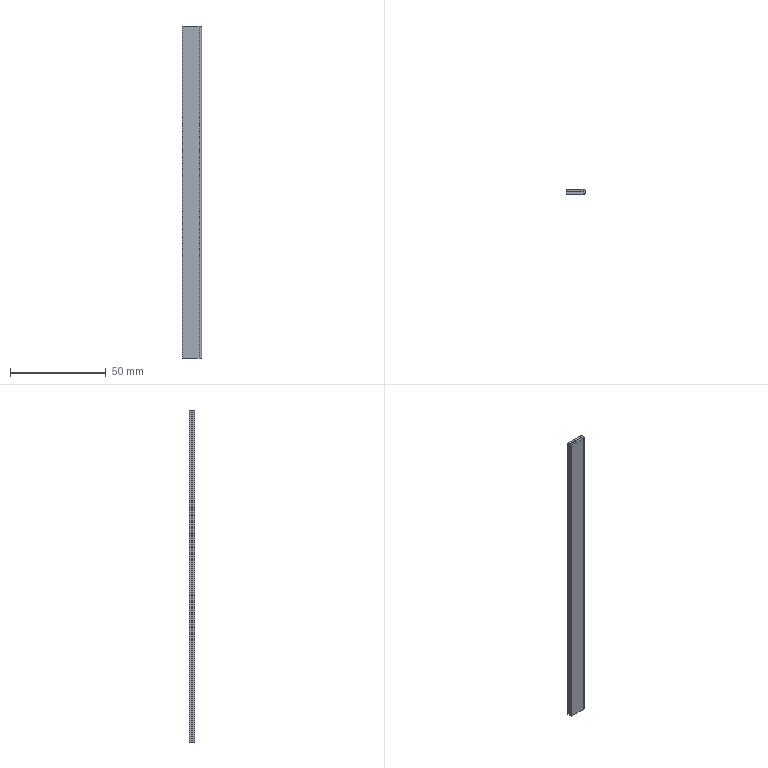Part | SolidWorks | features FlatPattern 1, Hem 1, ICE 1, SMBaseFlange 1, SheetMetal 1 | 1 solid | 12 faces | box 10 x 2.7 x 173.1 mm | volume 4083 mm3 | plane 10 | cylinder 2 | commonest cylinder face diameters 0.3 x1 2.7 x1
STEP:
#1=CARTESIAN_POINT('',(-12.962,-1.2,198.4));
#2=VERTEX_POINT('',#1);
#3=CARTESIAN_POINT('',(-12.962,-1.2,25.3));
#4=VERTEX_POINT('',#3);
#5=CARTESIAN_POINT('',(-12.962,-1.2,198.4));
#6=DIRECTION('',(0.,0.,-1.));
#7=VECTOR('',#6,1000.);
#8=LINE('',#5,#7);
#9=EDGE_CURVE('',#2,#4,#8,.T.);
#10=ORIENTED_EDGE('',*,*,#9,.T.);
#11=CARTESIAN_POINT('',(-4.312,-1.2,25.3));
#12=VERTEX_POINT('',#11);
#13=CARTESIAN_POINT('',(-12.962,-1.2,25.3));
#14=DIRECTION('',(1.,0.,0.));
#15=VECTOR('',#14,1000.);
#16=LINE('',#13,#15);
#17=EDGE_CURVE('',#4,#12,#16,.T.);
#18=ORIENTED_EDGE('',*,*,#17,.T.);
#19=CARTESIAN_POINT('',(-4.312,-1.2,198.4));
#20=VERTEX_POINT('',#19);
#21=CARTESIAN_POINT('',(-4.312,-1.2,0.));
#22=DIRECTION('',(0.,0.,1.));
#23=VECTOR('',#22,1000.);
#24=LINE('',#21,#23);
#25=EDGE_CURVE('',#12,#20,#24,.T.);
#26=ORIENTED_EDGE('',*,*,#25,.T.);
#27=CARTESIAN_POINT('',(-12.962,-1.2,198.4));
#28=DIRECTION('',(1.,0.,0.));
#29=VECTOR('',#28,1000.);
#30=LINE('',#27,#29);
#31=EDGE_CURVE('',#2,#20,#30,.T.);
#32=ORIENTED_EDGE('',*,*,#31,.F.);
#33=EDGE_LOOP('',(#10,#18,#26,#32));
#34=FACE_OUTER_BOUND('',#33,.T.);
#35=CARTESIAN_POINT('',(-12.962,-1.2,198.4));
#36=DIRECTION('',(0.,1.,0.));
#37=DIRECTION('',(0.,0.,1.));
#38=AXIS2_PLACEMENT_3D('',#35,#36,#37);
#39=PLANE('',#38);
#40=ADVANCED_FACE('',(#34),#39,.F.);
#41=CARTESIAN_POINT('',(-12.962,0.,25.3));
#42=VERTEX_POINT('',#41);
#43=CARTESIAN_POINT('',(-4.312,0.,25.3));
#44=VERTEX_POINT('',#43);
#45=CARTESIAN_POINT('',(-12.962,0.,25.3));
#46=DIRECTION('',(1.,0.,0.));
#47=VECTOR('',#46,1000.);
#48=LINE('',#45,#47);
#49=EDGE_CURVE('',#42,#44,#48,.T.);
#50=ORIENTED_EDGE('',*,*,#49,.F.);
#51=CARTESIAN_POINT('',(-12.962,0.,198.4));
#52=VERTEX_POINT('',#51);
#53=CARTESIAN_POINT('',(-12.962,0.,198.4));
#54=DIRECTION('',(0.,0.,-1.));
#55=VECTOR('',#54,1000.);
#56=LINE('',#53,#55);
#57=EDGE_CURVE('',#52,#42,#56,.T.);
#58=ORIENTED_EDGE('',*,*,#57,.F.);
#59=CARTESIAN_POINT('',(-4.312,0.,198.4));
#60=VERTEX_POINT('',#59);
#61=CARTESIAN_POINT('',(-12.962,0.,198.4));
#62=DIRECTION('',(1.,0.,0.));
#63=VECTOR('',#62,1000.);
#64=LINE('',#61,#63);
#65=EDGE_CURVE('',#52,#60,#64,.T.);
#66=ORIENTED_EDGE('',*,*,#65,.T.);
#67=CARTESIAN_POINT('',(-4.312,0.,0.));
#68=DIRECTION('',(0.,0.,1.));
#69=VECTOR('',#68,1000.);
#70=LINE('',#67,#69);
#71=EDGE_CURVE('',#44,#60,#70,.T.);
#72=ORIENTED_EDGE('',*,*,#71,.F.);
#73=EDGE_LOOP('',(#50,#58,#66,#72));
#74=FACE_OUTER_BOUND('',#73,.T.);
#75=CARTESIAN_POINT('',(-12.962,0.,198.4));
#76=DIRECTION('',(0.,1.,0.));
#77=DIRECTION('',(0.,0.,1.));
#78=AXIS2_PLACEMENT_3D('',#75,#76,#77);
#79=PLANE('',#78);
#80=ADVANCED_FACE('',(#74),#79,.T.);
#81=CARTESIAN_POINT('',(-12.962,-1.2,25.3));
#82=DIRECTION('',(0.,1.,0.));
#83=VECTOR('',#82,1000.);
#84=LINE('',#81,#83);
#85=EDGE_CURVE('',#4,#42,#84,.T.);
#86=ORIENTED_EDGE('',*,*,#85,.F.);
#87=ORIENTED_EDGE('',*,*,#9,.F.);
#88=CARTESIAN_POINT('',(-12.962,-1.2,198.4));
#89=DIRECTION('',(0.,1.,0.));
#90=VECTOR('',#89,1000.);
#91=LINE('',#88,#90);
#92=EDGE_CURVE('',#2,#52,#91,.T.);
#93=ORIENTED_EDGE('',*,*,#92,.T.);
#94=ORIENTED_EDGE('',*,*,#57,.T.);
#95=EDGE_LOOP('',(#86,#87,#93,#94));
#96=FACE_OUTER_BOUND('',#95,.T.);
#97=CARTESIAN_POINT('',(-12.962,-1.2,198.4));
#98=DIRECTION('',(-1.,0.,0.));
#99=DIRECTION('',(0.,0.,1.));
#100=AXIS2_PLACEMENT_3D('',#97,#98,#99);
#101=PLANE('',#100);
#102=ADVANCED_FACE('',(#96),#101,.T.);
#103=ORIENTED_EDGE('',*,*,#31,.T.);
#104=CARTESIAN_POINT('',(-4.312,0.,198.4));
#105=DIRECTION('',(0.,-1.,0.));
#106=VECTOR('',#105,1000.);
#107=LINE('',#104,#106);
#108=EDGE_CURVE('',#60,#20,#107,.T.);
#109=ORIENTED_EDGE('',*,*,#108,.F.);
#110=ORIENTED_EDGE('',*,*,#65,.F.);
#111=ORIENTED_EDGE('',*,*,#92,.F.);
#112=EDGE_LOOP('',(#103,#109,#110,#111));
#113=FACE_OUTER_BOUND('',#112,.T.);
#114=CARTESIAN_POINT('',(0.,0.,198.4));
#115=DIRECTION('',(0.,0.,-1.));
#116=DIRECTION('',(-1.,0.,0.));
#117=AXIS2_PLACEMENT_3D('',#114,#115,#116);
#118=PLANE('',#117);
#119=ADVANCED_FACE('',(#113),#118,.F.);
#120=CARTESIAN_POINT('',(-12.962,0.3,25.3));
#121=VERTEX_POINT('',#120);
#122=CARTESIAN_POINT('',(-12.962,1.5,25.3));
#123=VERTEX_POINT('',#122);
#124=CARTESIAN_POINT('',(-12.962,1.5,25.3));
#125=DIRECTION('',(0.,1.,0.));
#126=VECTOR('',#125,1000.);
#127=LINE('',#124,#126);
#128=EDGE_CURVE('',#121,#123,#127,.T.);
#129=ORIENTED_EDGE('',*,*,#128,.F.);
#130=CARTESIAN_POINT('',(-12.962,0.3,198.4));
#131=VERTEX_POINT('',#130);
#132=CARTESIAN_POINT('',(-12.962,0.3,99.2));
#133=DIRECTION('',(0.,0.,-1.));
#134=VECTOR('',#133,1000.);
#135=LINE('',#132,#134);
#136=EDGE_CURVE('',#131,#121,#135,.T.);
#137=ORIENTED_EDGE('',*,*,#136,.F.);
#138=CARTESIAN_POINT('',(-12.962,1.5,198.4));
#139=VERTEX_POINT('',#138);
#140=CARTESIAN_POINT('',(-12.962,1.5,198.4));
#141=DIRECTION('',(0.,1.,0.));
#142=VECTOR('',#141,1000.);
#143=LINE('',#140,#142);
#144=EDGE_CURVE('',#131,#139,#143,.T.);
#145=ORIENTED_EDGE('',*,*,#144,.T.);
#146=CARTESIAN_POINT('',(-12.962,1.5,99.2));
#147=DIRECTION('',(0.,0.,-1.));
#148=VECTOR('',#147,1000.);
#149=LINE('',#146,#148);
#150=EDGE_CURVE('',#139,#123,#149,.T.);
#151=ORIENTED_EDGE('',*,*,#150,.T.);
#152=EDGE_LOOP('',(#129,#137,#145,#151));
#153=FACE_OUTER_BOUND('',#152,.T.);
#154=CARTESIAN_POINT('',(-12.962,1.5,99.2));
#155=DIRECTION('',(1.,0.,0.));
#156=DIRECTION('',(0.,0.,-1.));
#157=AXIS2_PLACEMENT_3D('',#154,#155,#156);
#158=PLANE('',#157);
#159=ADVANCED_FACE('',(#153),#158,.F.);
#160=CARTESIAN_POINT('',(-4.312,0.3,198.4));
#161=VERTEX_POINT('',#160);
#162=CARTESIAN_POINT('',(-8.637,0.3,198.4));
#163=DIRECTION('',(-1.,0.,0.));
#164=VECTOR('',#163,1000.);
#165=LINE('',#162,#164);
#166=EDGE_CURVE('',#161,#131,#165,.T.);
#167=ORIENTED_EDGE('',*,*,#166,.F.);
#168=CARTESIAN_POINT('',(-4.312,1.5,198.4));
#169=VERTEX_POINT('',#168);
#170=CARTESIAN_POINT('',(-4.312,1.5,198.4));
#171=DIRECTION('',(0.,1.,0.));
#172=VECTOR('',#171,1000.);
#173=LINE('',#170,#172);
#174=EDGE_CURVE('',#161,#169,#173,.T.);
#175=ORIENTED_EDGE('',*,*,#174,.T.);
#176=CARTESIAN_POINT('',(-8.637,1.5,198.4));
#177=DIRECTION('',(-1.,0.,0.));
#178=VECTOR('',#177,1000.);
#179=LINE('',#176,#178);
#180=EDGE_CURVE('',#169,#139,#179,.T.);
#181=ORIENTED_EDGE('',*,*,#180,.T.);
#182=ORIENTED_EDGE('',*,*,#144,.F.);
#183=EDGE_LOOP('',(#167,#175,#181,#182));
#184=FACE_OUTER_BOUND('',#183,.T.);
#185=CARTESIAN_POINT('',(-8.637,1.5,198.4));
#186=DIRECTION('',(0.,0.,-1.));
#187=DIRECTION('',(-1.,0.,0.));
#188=AXIS2_PLACEMENT_3D('',#185,#186,#187);
#189=PLANE('',#188);
#190=ADVANCED_FACE('',(#184),#189,.F.);
#191=CARTESIAN_POINT('',(-4.312,1.5,25.3));
#192=VERTEX_POINT('',#191);
#193=CARTESIAN_POINT('',(9.896,1.5,25.3));
#194=DIRECTION('',(1.,0.,0.));
#195=VECTOR('',#194,1000.);
#196=LINE('',#193,#195);
#197=EDGE_CURVE('',#123,#192,#196,.T.);
#198=ORIENTED_EDGE('',*,*,#197,.F.);
#199=ORIENTED_EDGE('',*,*,#150,.F.);
#200=ORIENTED_EDGE('',*,*,#180,.F.);
#201=CARTESIAN_POINT('',(-4.312,1.5,99.2));
#202=DIRECTION('',(0.,0.,1.));
#203=VECTOR('',#202,1000.);
#204=LINE('',#201,#203);
#205=EDGE_CURVE('',#192,#169,#204,.T.);
#206=ORIENTED_EDGE('',*,*,#205,.F.);
#207=EDGE_LOOP('',(#198,#199,#200,#206));
#208=FACE_OUTER_BOUND('',#207,.T.);
#209=CARTESIAN_POINT('',(-8.637,1.5,99.2));
#210=DIRECTION('',(0.,1.,0.));
#211=DIRECTION('',(0.,0.,1.));
#212=AXIS2_PLACEMENT_3D('',#209,#210,#211);
#213=PLANE('',#212);
#214=ADVANCED_FACE('',(#208),#213,.T.);
#215=ORIENTED_EDGE('',*,*,#136,.T.);
#216=CARTESIAN_POINT('',(-4.312,0.3,25.3));
#217=VERTEX_POINT('',#216);
#218=CARTESIAN_POINT('',(-8.637,0.3,25.3));
#219=DIRECTION('',(1.,0.,0.));
#220=VECTOR('',#219,1000.);
#221=LINE('',#218,#220);
#222=EDGE_CURVE('',#121,#217,#221,.T.);
#223=ORIENTED_EDGE('',*,*,#222,.T.);
#224=CARTESIAN_POINT('',(-4.312,0.3,99.2));
#225=DIRECTION('',(0.,0.,1.));
#226=VECTOR('',#225,1000.);
#227=LINE('',#224,#226);
#228=EDGE_CURVE('',#217,#161,#227,.T.);
#229=ORIENTED_EDGE('',*,*,#228,.T.);
#230=ORIENTED_EDGE('',*,*,#166,.T.);
#231=EDGE_LOOP('',(#215,#223,#229,#230));
#232=FACE_OUTER_BOUND('',#231,.T.);
#233=CARTESIAN_POINT('',(-8.637,0.3,99.2));
#234=DIRECTION('',(0.,1.,0.));
#235=DIRECTION('',(0.,0.,1.));
#236=AXIS2_PLACEMENT_3D('',#233,#234,#235);
#237=PLANE('',#236);
#238=ADVANCED_FACE('',(#232),#237,.F.);
#239=ORIENTED_EDGE('',*,*,#174,.F.);
#240=CARTESIAN_POINT('',(-4.312,0.15,198.4));
#241=DIRECTION('',(0.,0.,1.));
#242=DIRECTION('',(-1.,0.,0.));
#243=AXIS2_PLACEMENT_3D('',#240,#241,#242);
#244=CIRCLE('',#243,0.15);
#245=EDGE_CURVE('',#60,#161,#244,.T.);
#246=ORIENTED_EDGE('',*,*,#245,.F.);
#247=ORIENTED_EDGE('',*,*,#108,.T.);
#248=CARTESIAN_POINT('',(-4.312,0.15,198.4));
#249=DIRECTION('',(0.,0.,1.));
#250=DIRECTION('',(-1.,0.,0.));
#251=AXIS2_PLACEMENT_3D('',#248,#249,#250);
#252=CIRCLE('',#251,1.35);
#253=EDGE_CURVE('',#20,#169,#252,.T.);
#254=ORIENTED_EDGE('',*,*,#253,.T.);
#255=EDGE_LOOP('',(#239,#246,#247,#254));
#256=FACE_OUTER_BOUND('',#255,.T.);
#257=CARTESIAN_POINT('',(-4.312,0.15,198.4));
#258=DIRECTION('',(0.,0.,1.));
#259=DIRECTION('',(1.,0.,0.));
#260=AXIS2_PLACEMENT_3D('',#257,#258,#259);
#261=PLANE('',#260);
#262=ADVANCED_FACE('',(#256),#261,.T.);
#263=CARTESIAN_POINT('',(-4.312,0.15,25.3));
#264=DIRECTION('',(0.,0.,-1.));
#265=DIRECTION('',(1.,0.,0.));
#266=AXIS2_PLACEMENT_3D('',#263,#264,#265);
#267=CIRCLE('',#266,1.35);
#268=EDGE_CURVE('',#192,#12,#267,.T.);
#269=ORIENTED_EDGE('',*,*,#268,.F.);
#270=ORIENTED_EDGE('',*,*,#205,.T.);
#271=ORIENTED_EDGE('',*,*,#253,.F.);
#272=ORIENTED_EDGE('',*,*,#25,.F.);
#273=EDGE_LOOP('',(#269,#270,#271,#272));
#274=FACE_OUTER_BOUND('',#273,.T.);
#275=CARTESIAN_POINT('',(-4.312,0.15,0.));
#276=DIRECTION('',(0.,0.,-1.));
#277=DIRECTION('',(0.,1.,0.));
#278=AXIS2_PLACEMENT_3D('',#275,#276,#277);
#279=CYLINDRICAL_SURFACE('',#278,1.35);
#280=ADVANCED_FACE('',(#274),#279,.T.);
#281=ORIENTED_EDGE('',*,*,#228,.F.);
#282=CARTESIAN_POINT('',(-4.312,0.15,25.3));
#283=DIRECTION('',(0.,0.,-1.));
#284=DIRECTION('',(1.,0.,0.));
#285=AXIS2_PLACEMENT_3D('',#282,#283,#284);
#286=CIRCLE('',#285,0.15);
#287=EDGE_CURVE('',#217,#44,#286,.T.);
#288=ORIENTED_EDGE('',*,*,#287,.T.);
#289=ORIENTED_EDGE('',*,*,#71,.T.);
#290=ORIENTED_EDGE('',*,*,#245,.T.);
#291=EDGE_LOOP('',(#281,#288,#289,#290));
#292=FACE_OUTER_BOUND('',#291,.T.);
#293=CARTESIAN_POINT('',(-4.312,0.15,0.));
#294=DIRECTION('',(0.,0.,-1.));
#295=DIRECTION('',(0.,1.,0.));
#296=AXIS2_PLACEMENT_3D('',#293,#294,#295);
#297=CYLINDRICAL_SURFACE('',#296,0.15);
#298=ADVANCED_FACE('',(#292),#297,.F.);
#299=ORIENTED_EDGE('',*,*,#268,.T.);
#300=ORIENTED_EDGE('',*,*,#17,.F.);
#301=ORIENTED_EDGE('',*,*,#85,.T.);
#302=ORIENTED_EDGE('',*,*,#49,.T.);
#303=ORIENTED_EDGE('',*,*,#287,.F.);
#304=ORIENTED_EDGE('',*,*,#222,.F.);
#305=ORIENTED_EDGE('',*,*,#128,.T.);
#306=ORIENTED_EDGE('',*,*,#197,.T.);
#307=EDGE_LOOP('',(#299,#300,#301,#302,#303,#304,#305,#306));
#308=FACE_OUTER_BOUND('',#307,.T.);
#309=CARTESIAN_POINT('',(9.896,-11.,25.3));
#310=DIRECTION('',(0.,0.,1.));
#311=DIRECTION('',(1.,0.,0.));
#312=AXIS2_PLACEMENT_3D('',#309,#310,#311);
#313=PLANE('',#312);
#314=ADVANCED_FACE('',(#308),#313,.F.);
#315=CLOSED_SHELL('',(#40,#80,#102,#119,#159,#190,#214,#238,#262,#280,#298,#314));
#316=MANIFOLD_SOLID_BREP('',#315);
#317=CARTESIAN_POINT('',(0.,0.,0.));
#318=DIRECTION('',(0.,0.,1.));
#319=DIRECTION('',(1.,0.,0.));
#320=AXIS2_PLACEMENT_3D('',#317,#318,#319);
#321=(LENGTH_UNIT()NAMED_UNIT(*)SI_UNIT(.MILLI.,.METRE.));
#322=UNCERTAINTY_MEASURE_WITH_UNIT(LENGTH_MEASURE(0.00001),#321,'','');
#323=(NAMED_UNIT(*)PLANE_ANGLE_UNIT()SI_UNIT($,.RADIAN.));
#324=(NAMED_UNIT(*)SI_UNIT($,.STERADIAN.)SOLID_ANGLE_UNIT());
#325=(GEOMETRIC_REPRESENTATION_CONTEXT(3)GLOBAL_UNCERTAINTY_ASSIGNED_CONTEXT((#322))GLOBAL_UNIT_ASSIGNED_CONTEXT((#321,#323,#324))REPRESENTATION_CONTEXT('',''));
#326=ADVANCED_BREP_SHAPE_REPRESENTATION('',(#316,#320),#325);